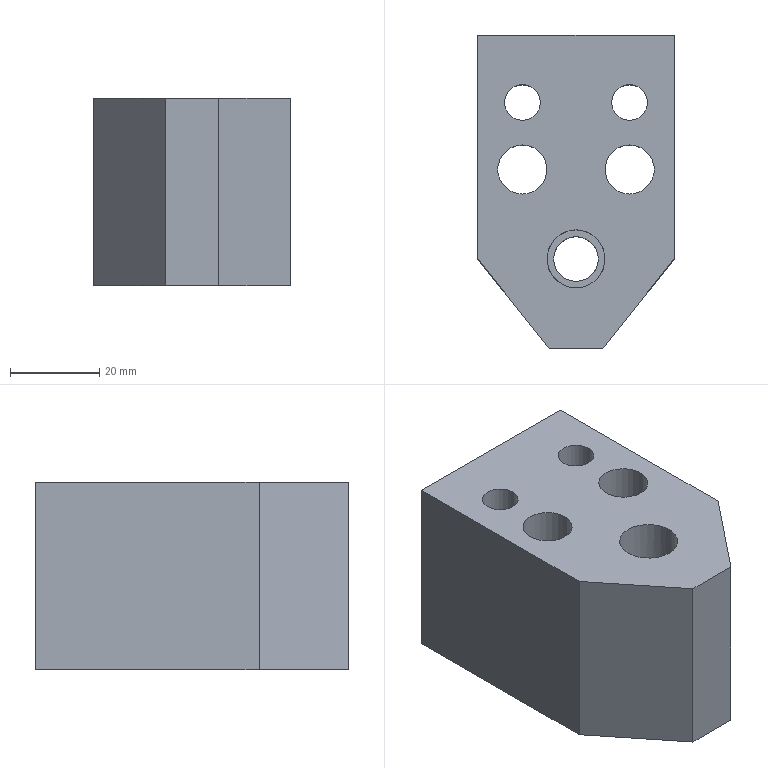Part | NX | features solid 2 | 1 solid | 19 faces | box 44 x 70 x 42 mm | volume 96430 mm3 | plane 11 | cylinder 8 | commonest cylinder face diameters 8 x2 11 x2 17 x2 10 x1 13 x1
STEP:
#1=CARTESIAN_POINT('',(-200.315,-13.728,113.));
#2=VERTEX_POINT('',#1);
#3=CARTESIAN_POINT('',(-200.315,-18.728,113.));
#4=DIRECTION('',(0.,0.,1.));
#5=DIRECTION('',(0.,1.,0.));
#6=AXIS2_PLACEMENT_3D('',#3,#4,#5);
#7=CIRCLE('',#6,5.);
#8=EDGE_CURVE('',#2,#2,#7,.F.);
#9=ORIENTED_EDGE('',*,*,#8,.F.);
#10=EDGE_LOOP('',(#9));
#11=FACE_BOUND('',#10,.T.);
#12=CARTESIAN_POINT('',(-212.315,-7.228,113.));
#13=VERTEX_POINT('',#12);
#14=CARTESIAN_POINT('',(-212.315,1.272,113.));
#15=DIRECTION('',(0.,0.,1.));
#16=DIRECTION('',(0.,-1.,0.));
#17=AXIS2_PLACEMENT_3D('',#14,#15,#16);
#18=CIRCLE('',#17,8.5);
#19=EDGE_CURVE('',#13,#13,#18,.T.);
#20=ORIENTED_EDGE('',*,*,#19,.T.);
#21=EDGE_LOOP('',(#20));
#22=FACE_BOUND('',#21,.T.);
#23=CARTESIAN_POINT('',(-188.315,-7.228,113.));
#24=VERTEX_POINT('',#23);
#25=CARTESIAN_POINT('',(-188.315,1.272,113.));
#26=DIRECTION('',(0.,0.,1.));
#27=DIRECTION('',(0.,-1.,0.));
#28=AXIS2_PLACEMENT_3D('',#25,#26,#27);
#29=CIRCLE('',#28,8.5);
#30=EDGE_CURVE('',#24,#24,#29,.T.);
#31=ORIENTED_EDGE('',*,*,#30,.T.);
#32=EDGE_LOOP('',(#31));
#33=FACE_BOUND('',#32,.T.);
#34=CARTESIAN_POINT('',(-212.315,12.272,113.));
#35=VERTEX_POINT('',#34);
#36=CARTESIAN_POINT('',(-212.315,16.272,113.));
#37=DIRECTION('',(0.,0.,1.));
#38=DIRECTION('',(0.,-1.,0.));
#39=AXIS2_PLACEMENT_3D('',#36,#37,#38);
#40=CIRCLE('',#39,4.);
#41=EDGE_CURVE('',#35,#35,#40,.T.);
#42=ORIENTED_EDGE('',*,*,#41,.T.);
#43=EDGE_LOOP('',(#42));
#44=FACE_BOUND('',#43,.T.);
#45=CARTESIAN_POINT('',(-188.315,12.272,113.));
#46=VERTEX_POINT('',#45);
#47=CARTESIAN_POINT('',(-188.315,16.272,113.));
#48=DIRECTION('',(0.,0.,1.));
#49=DIRECTION('',(0.,-1.,0.));
#50=AXIS2_PLACEMENT_3D('',#47,#48,#49);
#51=CIRCLE('',#50,4.);
#52=EDGE_CURVE('',#46,#46,#51,.T.);
#53=ORIENTED_EDGE('',*,*,#52,.T.);
#54=EDGE_LOOP('',(#53));
#55=FACE_BOUND('',#54,.T.);
#56=CARTESIAN_POINT('',(-194.315,-38.728,113.));
#57=VERTEX_POINT('',#56);
#58=CARTESIAN_POINT('',(-178.315,-18.728,113.));
#59=VERTEX_POINT('',#58);
#60=CARTESIAN_POINT('',(-155.388,9.931,113.));
#61=DIRECTION('',(0.6247,0.7809,0.));
#62=VECTOR('',#61,1000.);
#63=LINE('',#60,#62);
#64=EDGE_CURVE('',#57,#59,#63,.T.);
#65=ORIENTED_EDGE('',*,*,#64,.F.);
#66=CARTESIAN_POINT('',(-206.315,-38.728,113.));
#67=VERTEX_POINT('',#66);
#68=CARTESIAN_POINT('',(-200.315,-38.728,113.));
#69=DIRECTION('',(1.,0.,0.));
#70=VECTOR('',#69,1000.);
#71=LINE('',#68,#70);
#72=EDGE_CURVE('',#67,#57,#71,.T.);
#73=ORIENTED_EDGE('',*,*,#72,.F.);
#74=CARTESIAN_POINT('',(-222.315,-18.728,113.));
#75=VERTEX_POINT('',#74);
#76=CARTESIAN_POINT('',(-228.071,-11.533,113.));
#77=DIRECTION('',(-0.6247,0.7809,0.));
#78=VECTOR('',#77,1000.);
#79=LINE('',#76,#78);
#80=EDGE_CURVE('',#67,#75,#79,.T.);
#81=ORIENTED_EDGE('',*,*,#80,.T.);
#82=CARTESIAN_POINT('',(-222.315,31.272,113.));
#83=VERTEX_POINT('',#82);
#84=CARTESIAN_POINT('',(-222.315,-21.728,113.));
#85=DIRECTION('',(0.,1.,0.));
#86=VECTOR('',#85,1000.);
#87=LINE('',#84,#86);
#88=EDGE_CURVE('',#75,#83,#87,.T.);
#89=ORIENTED_EDGE('',*,*,#88,.T.);
#90=CARTESIAN_POINT('',(-178.315,31.272,113.));
#91=VERTEX_POINT('',#90);
#92=CARTESIAN_POINT('',(-178.315,31.272,113.));
#93=DIRECTION('',(-1.,0.,0.));
#94=VECTOR('',#93,1000.);
#95=LINE('',#92,#94);
#96=EDGE_CURVE('',#91,#83,#95,.T.);
#97=ORIENTED_EDGE('',*,*,#96,.F.);
#98=CARTESIAN_POINT('',(-178.315,-21.728,113.));
#99=DIRECTION('',(0.,1.,0.));
#100=VECTOR('',#99,1000.);
#101=LINE('',#98,#100);
#102=EDGE_CURVE('',#59,#91,#101,.T.);
#103=ORIENTED_EDGE('',*,*,#102,.F.);
#104=EDGE_LOOP('',(#65,#73,#81,#89,#97,#103));
#105=FACE_BOUND('',#104,.T.);
#106=CARTESIAN_POINT('',(-178.315,28.272,113.));
#107=DIRECTION('',(0.,0.,1.));
#108=DIRECTION('',(0.,-1.,0.));
#109=AXIS2_PLACEMENT_3D('',#106,#107,#108);
#110=PLANE('',#109);
#111=ADVANCED_FACE('',(#11,#22,#33,#44,#55,#105),#110,.F.);
#112=CARTESIAN_POINT('',(-178.315,-18.728,155.));
#113=VERTEX_POINT('',#112);
#114=CARTESIAN_POINT('',(-178.315,31.272,155.));
#115=VERTEX_POINT('',#114);
#116=CARTESIAN_POINT('',(-178.315,28.272,155.));
#117=DIRECTION('',(0.,1.,0.));
#118=VECTOR('',#117,1000.);
#119=LINE('',#116,#118);
#120=EDGE_CURVE('',#113,#115,#119,.T.);
#121=ORIENTED_EDGE('',*,*,#120,.F.);
#122=CARTESIAN_POINT('',(-178.315,-18.728,53.));
#123=DIRECTION('',(0.,0.,1.));
#124=VECTOR('',#123,1000.);
#125=LINE('',#122,#124);
#126=EDGE_CURVE('',#59,#113,#125,.T.);
#127=ORIENTED_EDGE('',*,*,#126,.F.);
#128=ORIENTED_EDGE('',*,*,#102,.T.);
#129=CARTESIAN_POINT('',(-178.315,31.272,113.));
#130=DIRECTION('',(0.,0.,1.));
#131=VECTOR('',#130,1000.);
#132=LINE('',#129,#131);
#133=EDGE_CURVE('',#91,#115,#132,.T.);
#134=ORIENTED_EDGE('',*,*,#133,.T.);
#135=EDGE_LOOP('',(#121,#127,#128,#134));
#136=FACE_BOUND('',#135,.T.);
#137=CARTESIAN_POINT('',(-178.315,-21.728,113.));
#138=DIRECTION('',(1.,0.,0.));
#139=DIRECTION('',(0.,1.,0.));
#140=AXIS2_PLACEMENT_3D('',#137,#138,#139);
#141=PLANE('',#140);
#142=ADVANCED_FACE('',(#136),#141,.T.);
#143=CARTESIAN_POINT('',(-188.315,20.272,155.));
#144=VERTEX_POINT('',#143);
#145=CARTESIAN_POINT('',(-188.315,16.272,155.));
#146=DIRECTION('',(0.,0.,1.));
#147=DIRECTION('',(0.,1.,0.));
#148=AXIS2_PLACEMENT_3D('',#145,#146,#147);
#149=CIRCLE('',#148,4.);
#150=EDGE_CURVE('',#144,#144,#149,.T.);
#151=ORIENTED_EDGE('',*,*,#150,.F.);
#152=EDGE_LOOP('',(#151));
#153=FACE_BOUND('',#152,.T.);
#154=CARTESIAN_POINT('',(-212.315,20.272,155.));
#155=VERTEX_POINT('',#154);
#156=CARTESIAN_POINT('',(-212.315,16.272,155.));
#157=DIRECTION('',(0.,0.,1.));
#158=DIRECTION('',(0.,1.,0.));
#159=AXIS2_PLACEMENT_3D('',#156,#157,#158);
#160=CIRCLE('',#159,4.);
#161=EDGE_CURVE('',#155,#155,#160,.T.);
#162=ORIENTED_EDGE('',*,*,#161,.F.);
#163=EDGE_LOOP('',(#162));
#164=FACE_BOUND('',#163,.T.);
#165=CARTESIAN_POINT('',(-188.315,6.772,155.));
#166=VERTEX_POINT('',#165);
#167=CARTESIAN_POINT('',(-188.315,1.272,155.));
#168=DIRECTION('',(0.,0.,1.));
#169=DIRECTION('',(0.,1.,0.));
#170=AXIS2_PLACEMENT_3D('',#167,#168,#169);
#171=CIRCLE('',#170,5.5);
#172=EDGE_CURVE('',#166,#166,#171,.T.);
#173=ORIENTED_EDGE('',*,*,#172,.F.);
#174=EDGE_LOOP('',(#173));
#175=FACE_BOUND('',#174,.T.);
#176=CARTESIAN_POINT('',(-212.315,6.772,155.));
#177=VERTEX_POINT('',#176);
#178=CARTESIAN_POINT('',(-212.315,1.272,155.));
#179=DIRECTION('',(0.,0.,1.));
#180=DIRECTION('',(0.,1.,0.));
#181=AXIS2_PLACEMENT_3D('',#178,#179,#180);
#182=CIRCLE('',#181,5.5);
#183=EDGE_CURVE('',#177,#177,#182,.T.);
#184=ORIENTED_EDGE('',*,*,#183,.F.);
#185=EDGE_LOOP('',(#184));
#186=FACE_BOUND('',#185,.T.);
#187=CARTESIAN_POINT('',(-200.315,-12.228,155.));
#188=VERTEX_POINT('',#187);
#189=CARTESIAN_POINT('',(-200.315,-18.728,155.));
#190=DIRECTION('',(0.,0.,1.));
#191=DIRECTION('',(0.,1.,0.));
#192=AXIS2_PLACEMENT_3D('',#189,#190,#191);
#193=CIRCLE('',#192,6.5);
#194=EDGE_CURVE('',#188,#188,#193,.T.);
#195=ORIENTED_EDGE('',*,*,#194,.F.);
#196=EDGE_LOOP('',(#195));
#197=FACE_BOUND('',#196,.T.);
#198=CARTESIAN_POINT('',(-206.315,-38.728,155.));
#199=VERTEX_POINT('',#198);
#200=CARTESIAN_POINT('',(-194.315,-38.728,155.));
#201=VERTEX_POINT('',#200);
#202=CARTESIAN_POINT('',(-178.315,-38.728,155.));
#203=DIRECTION('',(1.,0.,0.));
#204=VECTOR('',#203,1000.);
#205=LINE('',#202,#204);
#206=EDGE_CURVE('',#199,#201,#205,.T.);
#207=ORIENTED_EDGE('',*,*,#206,.T.);
#208=CARTESIAN_POINT('',(-155.388,9.931,155.));
#209=DIRECTION('',(0.6247,0.7809,0.));
#210=VECTOR('',#209,1000.);
#211=LINE('',#208,#210);
#212=EDGE_CURVE('',#201,#113,#211,.T.);
#213=ORIENTED_EDGE('',*,*,#212,.T.);
#214=ORIENTED_EDGE('',*,*,#120,.T.);
#215=CARTESIAN_POINT('',(-222.315,31.272,155.));
#216=VERTEX_POINT('',#215);
#217=CARTESIAN_POINT('',(-178.315,31.272,155.));
#218=DIRECTION('',(-1.,0.,0.));
#219=VECTOR('',#218,1000.);
#220=LINE('',#217,#219);
#221=EDGE_CURVE('',#115,#216,#220,.T.);
#222=ORIENTED_EDGE('',*,*,#221,.T.);
#223=CARTESIAN_POINT('',(-222.315,-18.728,155.));
#224=VERTEX_POINT('',#223);
#225=CARTESIAN_POINT('',(-222.315,28.272,155.));
#226=DIRECTION('',(0.,1.,0.));
#227=VECTOR('',#226,1000.);
#228=LINE('',#225,#227);
#229=EDGE_CURVE('',#224,#216,#228,.T.);
#230=ORIENTED_EDGE('',*,*,#229,.F.);
#231=CARTESIAN_POINT('',(-228.071,-11.533,155.));
#232=DIRECTION('',(-0.6247,0.7809,0.));
#233=VECTOR('',#232,1000.);
#234=LINE('',#231,#233);
#235=EDGE_CURVE('',#199,#224,#234,.T.);
#236=ORIENTED_EDGE('',*,*,#235,.F.);
#237=EDGE_LOOP('',(#207,#213,#214,#222,#230,#236));
#238=FACE_BOUND('',#237,.T.);
#239=CARTESIAN_POINT('',(-178.315,28.272,155.));
#240=DIRECTION('',(0.,0.,1.));
#241=DIRECTION('',(0.,-1.,0.));
#242=AXIS2_PLACEMENT_3D('',#239,#240,#241);
#243=PLANE('',#242);
#244=ADVANCED_FACE('',(#153,#164,#175,#186,#197,#238),#243,.T.);
#245=ORIENTED_EDGE('',*,*,#221,.F.);
#246=ORIENTED_EDGE('',*,*,#133,.F.);
#247=ORIENTED_EDGE('',*,*,#96,.T.);
#248=CARTESIAN_POINT('',(-222.315,31.272,113.));
#249=DIRECTION('',(0.,0.,1.));
#250=VECTOR('',#249,1000.);
#251=LINE('',#248,#250);
#252=EDGE_CURVE('',#83,#216,#251,.T.);
#253=ORIENTED_EDGE('',*,*,#252,.T.);
#254=EDGE_LOOP('',(#245,#246,#247,#253));
#255=FACE_BOUND('',#254,.T.);
#256=CARTESIAN_POINT('',(-178.315,31.272,113.));
#257=DIRECTION('',(0.,1.,0.));
#258=DIRECTION('',(-1.,0.,0.));
#259=AXIS2_PLACEMENT_3D('',#256,#257,#258);
#260=PLANE('',#259);
#261=ADVANCED_FACE('',(#255),#260,.T.);
#262=ORIENTED_EDGE('',*,*,#88,.F.);
#263=CARTESIAN_POINT('',(-222.315,-18.728,53.));
#264=DIRECTION('',(0.,0.,1.));
#265=VECTOR('',#264,1000.);
#266=LINE('',#263,#265);
#267=EDGE_CURVE('',#75,#224,#266,.T.);
#268=ORIENTED_EDGE('',*,*,#267,.T.);
#269=ORIENTED_EDGE('',*,*,#229,.T.);
#270=ORIENTED_EDGE('',*,*,#252,.F.);
#271=EDGE_LOOP('',(#262,#268,#269,#270));
#272=FACE_BOUND('',#271,.T.);
#273=CARTESIAN_POINT('',(-222.315,-21.728,113.));
#274=DIRECTION('',(1.,0.,0.));
#275=DIRECTION('',(0.,1.,0.));
#276=AXIS2_PLACEMENT_3D('',#273,#274,#275);
#277=PLANE('',#276);
#278=ADVANCED_FACE('',(#272),#277,.F.);
#279=ORIENTED_EDGE('',*,*,#206,.F.);
#280=CARTESIAN_POINT('',(-206.315,-38.728,113.));
#281=DIRECTION('',(0.,0.,1.));
#282=VECTOR('',#281,1000.);
#283=LINE('',#280,#282);
#284=EDGE_CURVE('',#67,#199,#283,.T.);
#285=ORIENTED_EDGE('',*,*,#284,.F.);
#286=ORIENTED_EDGE('',*,*,#72,.T.);
#287=CARTESIAN_POINT('',(-194.315,-38.728,113.));
#288=DIRECTION('',(0.,0.,1.));
#289=VECTOR('',#288,1000.);
#290=LINE('',#287,#289);
#291=EDGE_CURVE('',#57,#201,#290,.T.);
#292=ORIENTED_EDGE('',*,*,#291,.T.);
#293=EDGE_LOOP('',(#279,#285,#286,#292));
#294=FACE_BOUND('',#293,.T.);
#295=CARTESIAN_POINT('',(-200.315,-38.728,113.));
#296=DIRECTION('',(0.,-1.,0.));
#297=DIRECTION('',(1.,0.,0.));
#298=AXIS2_PLACEMENT_3D('',#295,#296,#297);
#299=PLANE('',#298);
#300=ADVANCED_FACE('',(#294),#299,.T.);
#301=ORIENTED_EDGE('',*,*,#150,.T.);
#302=EDGE_LOOP('',(#301));
#303=FACE_BOUND('',#302,.T.);
#304=ORIENTED_EDGE('',*,*,#52,.F.);
#305=EDGE_LOOP('',(#304));
#306=FACE_BOUND('',#305,.T.);
#307=CARTESIAN_POINT('',(-188.315,16.272,113.));
#308=DIRECTION('',(0.,0.,1.));
#309=DIRECTION('',(0.,-1.,0.));
#310=AXIS2_PLACEMENT_3D('',#307,#308,#309);
#311=CYLINDRICAL_SURFACE('',#310,4.);
#312=ADVANCED_FACE('',(#303,#306),#311,.F.);
#313=ORIENTED_EDGE('',*,*,#161,.T.);
#314=EDGE_LOOP('',(#313));
#315=FACE_BOUND('',#314,.T.);
#316=ORIENTED_EDGE('',*,*,#41,.F.);
#317=EDGE_LOOP('',(#316));
#318=FACE_BOUND('',#317,.T.);
#319=CARTESIAN_POINT('',(-212.315,16.272,113.));
#320=DIRECTION('',(0.,0.,1.));
#321=DIRECTION('',(0.,-1.,0.));
#322=AXIS2_PLACEMENT_3D('',#319,#320,#321);
#323=CYLINDRICAL_SURFACE('',#322,4.);
#324=ADVANCED_FACE('',(#315,#318),#323,.F.);
#325=ORIENTED_EDGE('',*,*,#172,.T.);
#326=EDGE_LOOP('',(#325));
#327=FACE_BOUND('',#326,.T.);
#328=CARTESIAN_POINT('',(-188.315,-4.228,124.));
#329=VERTEX_POINT('',#328);
#330=CARTESIAN_POINT('',(-188.315,1.272,124.));
#331=DIRECTION('',(0.,0.,1.));
#332=DIRECTION('',(0.,-1.,0.));
#333=AXIS2_PLACEMENT_3D('',#330,#331,#332);
#334=CIRCLE('',#333,5.5);
#335=EDGE_CURVE('',#329,#329,#334,.T.);
#336=ORIENTED_EDGE('',*,*,#335,.F.);
#337=EDGE_LOOP('',(#336));
#338=FACE_BOUND('',#337,.T.);
#339=CARTESIAN_POINT('',(-188.315,1.272,163.));
#340=DIRECTION('',(0.,0.,1.));
#341=DIRECTION('',(0.,-1.,0.));
#342=AXIS2_PLACEMENT_3D('',#339,#340,#341);
#343=CYLINDRICAL_SURFACE('',#342,5.5);
#344=ADVANCED_FACE('',(#327,#338),#343,.F.);
#345=ORIENTED_EDGE('',*,*,#335,.T.);
#346=EDGE_LOOP('',(#345));
#347=FACE_BOUND('',#346,.T.);
#348=CARTESIAN_POINT('',(-188.315,-7.228,124.));
#349=VERTEX_POINT('',#348);
#350=CARTESIAN_POINT('',(-188.315,1.272,124.));
#351=DIRECTION('',(0.,0.,1.));
#352=DIRECTION('',(0.,-1.,0.));
#353=AXIS2_PLACEMENT_3D('',#350,#351,#352);
#354=CIRCLE('',#353,8.5);
#355=EDGE_CURVE('',#349,#349,#354,.T.);
#356=ORIENTED_EDGE('',*,*,#355,.F.);
#357=EDGE_LOOP('',(#356));
#358=FACE_BOUND('',#357,.T.);
#359=CARTESIAN_POINT('',(-188.315,1.272,124.));
#360=DIRECTION('',(0.,0.,1.));
#361=DIRECTION('',(0.,-1.,0.));
#362=AXIS2_PLACEMENT_3D('',#359,#360,#361);
#363=PLANE('',#362);
#364=ADVANCED_FACE('',(#347,#358),#363,.F.);
#365=ORIENTED_EDGE('',*,*,#355,.T.);
#366=EDGE_LOOP('',(#365));
#367=FACE_BOUND('',#366,.T.);
#368=ORIENTED_EDGE('',*,*,#30,.F.);
#369=EDGE_LOOP('',(#368));
#370=FACE_BOUND('',#369,.T.);
#371=CARTESIAN_POINT('',(-188.315,1.272,113.));
#372=DIRECTION('',(0.,0.,1.));
#373=DIRECTION('',(0.,-1.,0.));
#374=AXIS2_PLACEMENT_3D('',#371,#372,#373);
#375=CYLINDRICAL_SURFACE('',#374,8.5);
#376=ADVANCED_FACE('',(#367,#370),#375,.F.);
#377=ORIENTED_EDGE('',*,*,#183,.T.);
#378=EDGE_LOOP('',(#377));
#379=FACE_BOUND('',#378,.T.);
#380=CARTESIAN_POINT('',(-212.315,-4.228,124.));
#381=VERTEX_POINT('',#380);
#382=CARTESIAN_POINT('',(-212.315,1.272,124.));
#383=DIRECTION('',(0.,0.,1.));
#384=DIRECTION('',(0.,-1.,0.));
#385=AXIS2_PLACEMENT_3D('',#382,#383,#384);
#386=CIRCLE('',#385,5.5);
#387=EDGE_CURVE('',#381,#381,#386,.T.);
#388=ORIENTED_EDGE('',*,*,#387,.F.);
#389=EDGE_LOOP('',(#388));
#390=FACE_BOUND('',#389,.T.);
#391=CARTESIAN_POINT('',(-212.315,1.272,163.));
#392=DIRECTION('',(0.,0.,1.));
#393=DIRECTION('',(0.,-1.,0.));
#394=AXIS2_PLACEMENT_3D('',#391,#392,#393);
#395=CYLINDRICAL_SURFACE('',#394,5.5);
#396=ADVANCED_FACE('',(#379,#390),#395,.F.);
#397=ORIENTED_EDGE('',*,*,#387,.T.);
#398=EDGE_LOOP('',(#397));
#399=FACE_BOUND('',#398,.T.);
#400=CARTESIAN_POINT('',(-212.315,-7.228,124.));
#401=VERTEX_POINT('',#400);
#402=CARTESIAN_POINT('',(-212.315,1.272,124.));
#403=DIRECTION('',(0.,0.,1.));
#404=DIRECTION('',(0.,-1.,0.));
#405=AXIS2_PLACEMENT_3D('',#402,#403,#404);
#406=CIRCLE('',#405,8.5);
#407=EDGE_CURVE('',#401,#401,#406,.T.);
#408=ORIENTED_EDGE('',*,*,#407,.F.);
#409=EDGE_LOOP('',(#408));
#410=FACE_BOUND('',#409,.T.);
#411=CARTESIAN_POINT('',(-212.315,1.272,124.));
#412=DIRECTION('',(0.,0.,1.));
#413=DIRECTION('',(0.,-1.,0.));
#414=AXIS2_PLACEMENT_3D('',#411,#412,#413);
#415=PLANE('',#414);
#416=ADVANCED_FACE('',(#399,#410),#415,.F.);
#417=ORIENTED_EDGE('',*,*,#407,.T.);
#418=EDGE_LOOP('',(#417));
#419=FACE_BOUND('',#418,.T.);
#420=ORIENTED_EDGE('',*,*,#19,.F.);
#421=EDGE_LOOP('',(#420));
#422=FACE_BOUND('',#421,.T.);
#423=CARTESIAN_POINT('',(-212.315,1.272,113.));
#424=DIRECTION('',(0.,0.,1.));
#425=DIRECTION('',(0.,-1.,0.));
#426=AXIS2_PLACEMENT_3D('',#423,#424,#425);
#427=CYLINDRICAL_SURFACE('',#426,8.5);
#428=ADVANCED_FACE('',(#419,#422),#427,.F.);
#429=CARTESIAN_POINT('',(-195.315,-18.728,135.));
#430=VERTEX_POINT('',#429);
#431=CARTESIAN_POINT('',(-200.315,-18.728,135.));
#432=DIRECTION('',(0.,0.,-1.));
#433=DIRECTION('',(1.,0.,0.));
#434=AXIS2_PLACEMENT_3D('',#431,#432,#433);
#435=CIRCLE('',#434,5.);
#436=EDGE_CURVE('',#430,#430,#435,.F.);
#437=ORIENTED_EDGE('',*,*,#436,.T.);
#438=EDGE_LOOP('',(#437));
#439=FACE_BOUND('',#438,.T.);
#440=ORIENTED_EDGE('',*,*,#8,.T.);
#441=EDGE_LOOP('',(#440));
#442=FACE_BOUND('',#441,.T.);
#443=CARTESIAN_POINT('',(-200.315,-18.728,153.));
#444=DIRECTION('',(0.,0.,-1.));
#445=DIRECTION('',(0.,-1.,0.));
#446=AXIS2_PLACEMENT_3D('',#443,#444,#445);
#447=CYLINDRICAL_SURFACE('',#446,5.);
#448=ADVANCED_FACE('',(#439,#442),#447,.F.);
#449=ORIENTED_EDGE('',*,*,#194,.T.);
#450=EDGE_LOOP('',(#449));
#451=FACE_BOUND('',#450,.T.);
#452=CARTESIAN_POINT('',(-193.815,-18.728,135.));
#453=VERTEX_POINT('',#452);
#454=CARTESIAN_POINT('',(-200.315,-18.728,135.));
#455=DIRECTION('',(0.,0.,-1.));
#456=DIRECTION('',(1.,0.,0.));
#457=AXIS2_PLACEMENT_3D('',#454,#455,#456);
#458=CIRCLE('',#457,6.5);
#459=EDGE_CURVE('',#453,#453,#458,.F.);
#460=ORIENTED_EDGE('',*,*,#459,.F.);
#461=EDGE_LOOP('',(#460));
#462=FACE_BOUND('',#461,.T.);
#463=CARTESIAN_POINT('',(-200.315,-18.728,148.));
#464=DIRECTION('',(0.,0.,1.));
#465=DIRECTION('',(0.,1.,0.));
#466=AXIS2_PLACEMENT_3D('',#463,#464,#465);
#467=CYLINDRICAL_SURFACE('',#466,6.5);
#468=ADVANCED_FACE('',(#451,#462),#467,.F.);
#469=ORIENTED_EDGE('',*,*,#459,.T.);
#470=EDGE_LOOP('',(#469));
#471=FACE_BOUND('',#470,.T.);
#472=ORIENTED_EDGE('',*,*,#436,.F.);
#473=EDGE_LOOP('',(#472));
#474=FACE_BOUND('',#473,.T.);
#475=CARTESIAN_POINT('',(-200.315,-18.728,135.));
#476=DIRECTION('',(0.,0.,-1.));
#477=DIRECTION('',(0.,-1.,0.));
#478=AXIS2_PLACEMENT_3D('',#475,#476,#477);
#479=PLANE('',#478);
#480=ADVANCED_FACE('',(#471,#474),#479,.F.);
#481=ORIENTED_EDGE('',*,*,#284,.T.);
#482=ORIENTED_EDGE('',*,*,#235,.T.);
#483=ORIENTED_EDGE('',*,*,#267,.F.);
#484=ORIENTED_EDGE('',*,*,#80,.F.);
#485=EDGE_LOOP('',(#481,#482,#483,#484));
#486=FACE_BOUND('',#485,.T.);
#487=CARTESIAN_POINT('',(-206.315,-38.728,53.));
#488=DIRECTION('',(0.7809,0.6247,0.));
#489=DIRECTION('',(-0.6247,0.7809,0.));
#490=AXIS2_PLACEMENT_3D('',#487,#488,#489);
#491=PLANE('',#490);
#492=ADVANCED_FACE('',(#486),#491,.F.);
#493=ORIENTED_EDGE('',*,*,#64,.T.);
#494=ORIENTED_EDGE('',*,*,#126,.T.);
#495=ORIENTED_EDGE('',*,*,#212,.F.);
#496=ORIENTED_EDGE('',*,*,#291,.F.);
#497=EDGE_LOOP('',(#493,#494,#495,#496));
#498=FACE_BOUND('',#497,.T.);
#499=CARTESIAN_POINT('',(-194.315,-38.728,53.));
#500=DIRECTION('',(0.7809,-0.6247,0.));
#501=DIRECTION('',(0.6247,0.7809,0.));
#502=AXIS2_PLACEMENT_3D('',#499,#500,#501);
#503=PLANE('',#502);
#504=ADVANCED_FACE('',(#498),#503,.T.);
#505=CLOSED_SHELL('',(#111,#142,#244,#261,#278,#300,#312,#324,#344,#364,#376,#396,#416,#428,#448,#468,#480,#492,#504));
#506=MANIFOLD_SOLID_BREP('',#505);
#507=(LENGTH_UNIT()NAMED_UNIT(*)SI_UNIT(.MILLI.,.METRE.));
#508=UNCERTAINTY_MEASURE_WITH_UNIT(LENGTH_MEASURE(0.00001),#507,'','');
#509=(NAMED_UNIT(*)PLANE_ANGLE_UNIT()SI_UNIT($,.RADIAN.));
#510=(NAMED_UNIT(*)SI_UNIT($,.STERADIAN.)SOLID_ANGLE_UNIT());
#511=(GEOMETRIC_REPRESENTATION_CONTEXT(3)GLOBAL_UNCERTAINTY_ASSIGNED_CONTEXT((#508))GLOBAL_UNIT_ASSIGNED_CONTEXT((#507,#509,#510))REPRESENTATION_CONTEXT('',''));
#512=ADVANCED_BREP_SHAPE_REPRESENTATION('',(#506),#511);